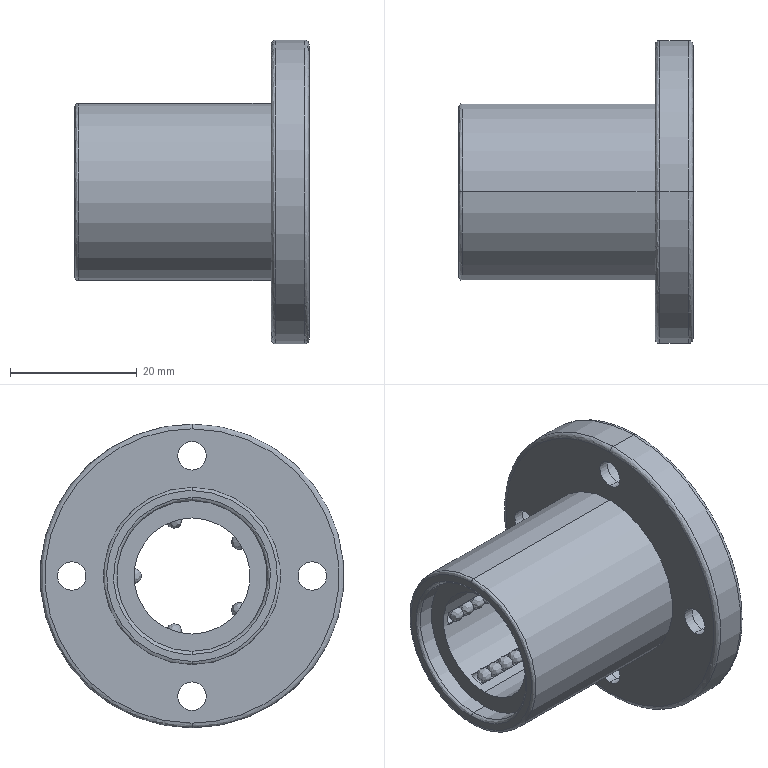Part | SolidWorks | features BaseBody 1 | 1 solid | 198 faces | box 37 x 48 x 48 mm | volume 18661 mm3 | spline 138 | cylinder 39 | plane 21 | commonest cylinder face diameters 2.35 x9 4.5 x8 8 x8 18.35 x2 19.2 x2 20.8 x2